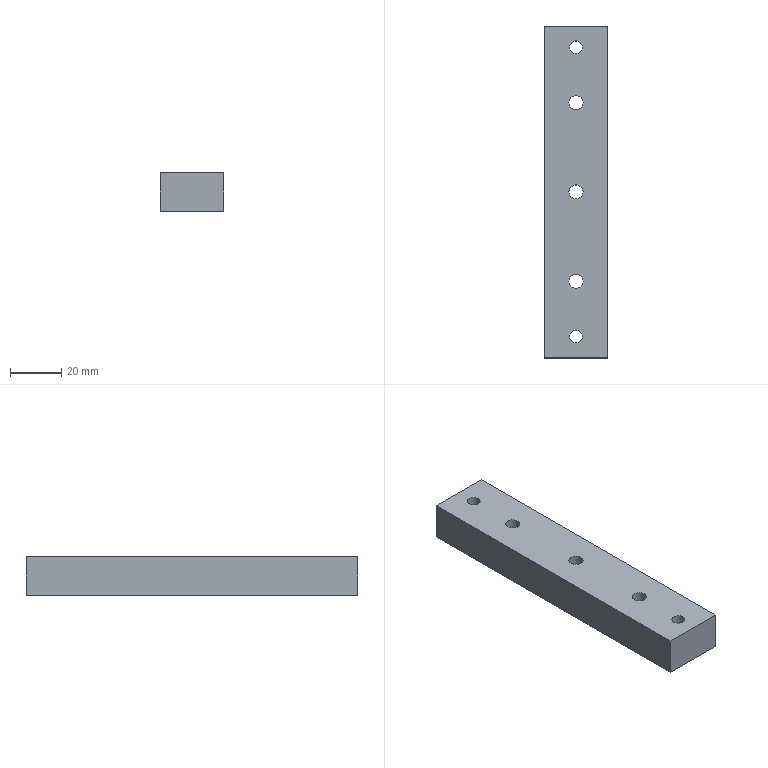Part | STEP file | 1 solid | 11 faces | box 25 x 130 x 15 mm | volume 47092 mm3 | plane 6 | cylinder 5 | commonest cylinder face diameters 5.5 x3 5 x2
STEP:
#1=CARTESIAN_POINT('',(0.,0.,0.));
#2=DIRECTION('',(0.,0.,1.));
#3=DIRECTION('',(1.,0.,0.));
#4=AXIS2_PLACEMENT_3D('',#1,#2,#3);
#5=CARTESIAN_POINT('',(1174.747,377.505,-51.381));
#6=VERTEX_POINT('',#5);
#7=CARTESIAN_POINT('',(1174.747,507.505,-51.381));
#8=VERTEX_POINT('',#7);
#9=CARTESIAN_POINT('',(1174.747,381.355,-51.381));
#10=DIRECTION('',(0.,1.,0.));
#11=VECTOR('',#10,1.);
#12=LINE('',#9,#11);
#13=CARTESIAN_POINT('',(1174.747,381.355,-48.381));
#14=DIRECTION('',(1.,0.,0.));
#15=DIRECTION('',(0.,0.,-1.));
#16=AXIS2_PLACEMENT_3D('',#13,#14,#15);
#17=PLANE('',#16);
#18=CARTESIAN_POINT('',(3.,0.));
#19=DIRECTION('',(0.,1.));
#20=VECTOR('',#19,1.);
#21=LINE('',#18,#20);
#22=(GEOMETRIC_REPRESENTATION_CONTEXT(2)PARAMETRIC_REPRESENTATION_CONTEXT()REPRESENTATION_CONTEXT('',''));
#23=DEFINITIONAL_REPRESENTATION('',(#21),#22);
#24=PCURVE('',#17,#23);
#25=CARTESIAN_POINT('',(18365.131,-3580.314,-51.381));
#26=DIRECTION('',(0.,0.,-1.));
#27=DIRECTION('',(-1.,0.,0.));
#28=AXIS2_PLACEMENT_3D('',#25,#26,#27);
#29=PLANE('',#28);
#30=CARTESIAN_POINT('',(17190.384,3961.669));
#31=DIRECTION('',(0.,1.));
#32=VECTOR('',#31,1.);
#33=LINE('',#30,#32);
#34=(GEOMETRIC_REPRESENTATION_CONTEXT(2)PARAMETRIC_REPRESENTATION_CONTEXT()REPRESENTATION_CONTEXT('',''));
#35=DEFINITIONAL_REPRESENTATION('',(#33),#34);
#36=PCURVE('',#29,#35);
#37=SURFACE_CURVE('',#12,(#24,#36),.PCURVE_S1.);
#38=EDGE_CURVE('',#6,#8,#37,.T.);
#39=ORIENTED_EDGE('',*,*,#38,.F.);
#40=CARTESIAN_POINT('',(1174.747,377.505,-36.381));
#41=VERTEX_POINT('',#40);
#42=CARTESIAN_POINT('',(1174.747,377.505,-48.381));
#43=DIRECTION('',(0.,0.,1.));
#44=VECTOR('',#43,1.);
#45=LINE('',#42,#44);
#46=CARTESIAN_POINT('',(0.,-3.85));
#47=DIRECTION('',(-1.,0.));
#48=VECTOR('',#47,1.);
#49=LINE('',#46,#48);
#50=(GEOMETRIC_REPRESENTATION_CONTEXT(2)PARAMETRIC_REPRESENTATION_CONTEXT()REPRESENTATION_CONTEXT('',''));
#51=DEFINITIONAL_REPRESENTATION('',(#49),#50);
#52=PCURVE('',#17,#51);
#53=CARTESIAN_POINT('',(1199.747,377.505,-48.381));
#54=DIRECTION('',(0.,1.,0.));
#55=DIRECTION('',(0.,0.,-1.));
#56=AXIS2_PLACEMENT_3D('',#53,#54,#55);
#57=PLANE('',#56);
#58=CARTESIAN_POINT('',(0.,25.));
#59=DIRECTION('',(-1.,0.));
#60=VECTOR('',#59,1.);
#61=LINE('',#58,#60);
#62=(GEOMETRIC_REPRESENTATION_CONTEXT(2)PARAMETRIC_REPRESENTATION_CONTEXT()REPRESENTATION_CONTEXT('',''));
#63=DEFINITIONAL_REPRESENTATION('',(#61),#62);
#64=PCURVE('',#57,#63);
#65=SURFACE_CURVE('',#45,(#52,#64),.PCURVE_S1.);
#66=EDGE_CURVE('',#6,#41,#65,.T.);
#67=ORIENTED_EDGE('',*,*,#66,.T.);
#68=CARTESIAN_POINT('',(1174.747,507.505,-36.381));
#69=VERTEX_POINT('',#68);
#70=CARTESIAN_POINT('',(1174.747,381.355,-36.381));
#71=DIRECTION('',(0.,1.,0.));
#72=VECTOR('',#71,1.);
#73=LINE('',#70,#72);
#74=CARTESIAN_POINT('',(-12.,0.));
#75=DIRECTION('',(0.,1.));
#76=VECTOR('',#75,1.);
#77=LINE('',#74,#76);
#78=(GEOMETRIC_REPRESENTATION_CONTEXT(2)PARAMETRIC_REPRESENTATION_CONTEXT()REPRESENTATION_CONTEXT('',''));
#79=DEFINITIONAL_REPRESENTATION('',(#77),#78);
#80=PCURVE('',#17,#79);
#81=CARTESIAN_POINT('',(18365.131,-3580.314,-36.381));
#82=DIRECTION('',(0.,0.,-1.));
#83=DIRECTION('',(-1.,0.,0.));
#84=AXIS2_PLACEMENT_3D('',#81,#82,#83);
#85=PLANE('',#84);
#86=CARTESIAN_POINT('',(17190.384,3961.669));
#87=DIRECTION('',(0.,1.));
#88=VECTOR('',#87,1.);
#89=LINE('',#86,#88);
#90=(GEOMETRIC_REPRESENTATION_CONTEXT(2)PARAMETRIC_REPRESENTATION_CONTEXT()REPRESENTATION_CONTEXT('',''));
#91=DEFINITIONAL_REPRESENTATION('',(#89),#90);
#92=PCURVE('',#85,#91);
#93=SURFACE_CURVE('',#73,(#80,#92),.PCURVE_S1.);
#94=EDGE_CURVE('',#41,#69,#93,.T.);
#95=ORIENTED_EDGE('',*,*,#94,.T.);
#96=CARTESIAN_POINT('',(1174.747,507.505,-48.381));
#97=DIRECTION('',(0.,0.,1.));
#98=VECTOR('',#97,1.);
#99=LINE('',#96,#98);
#100=CARTESIAN_POINT('',(0.,126.15));
#101=DIRECTION('',(-1.,0.));
#102=VECTOR('',#101,1.);
#103=LINE('',#100,#102);
#104=(GEOMETRIC_REPRESENTATION_CONTEXT(2)PARAMETRIC_REPRESENTATION_CONTEXT()REPRESENTATION_CONTEXT('',''));
#105=DEFINITIONAL_REPRESENTATION('',(#103),#104);
#106=PCURVE('',#17,#105);
#107=CARTESIAN_POINT('',(1174.747,507.505,-48.381));
#108=DIRECTION('',(0.,-1.,0.));
#109=DIRECTION('',(0.,0.,1.));
#110=AXIS2_PLACEMENT_3D('',#107,#108,#109);
#111=PLANE('',#110);
#112=CARTESIAN_POINT('',(0.,0.));
#113=DIRECTION('',(1.,0.));
#114=VECTOR('',#113,1.);
#115=LINE('',#112,#114);
#116=(GEOMETRIC_REPRESENTATION_CONTEXT(2)PARAMETRIC_REPRESENTATION_CONTEXT()REPRESENTATION_CONTEXT('',''));
#117=DEFINITIONAL_REPRESENTATION('',(#115),#116);
#118=PCURVE('',#111,#117);
#119=SURFACE_CURVE('',#99,(#106,#118),.PCURVE_S1.);
#120=EDGE_CURVE('',#8,#69,#119,.T.);
#121=ORIENTED_EDGE('',*,*,#120,.F.);
#122=EDGE_LOOP('',(#39,#67,#95,#121));
#123=FACE_BOUND('',#122,.T.);
#124=ADVANCED_FACE('',(#123),#17,.F.);
#125=CARTESIAN_POINT('',(1199.747,507.505,-36.381));
#126=VERTEX_POINT('',#125);
#127=CARTESIAN_POINT('',(1199.747,377.505,-36.381));
#128=VERTEX_POINT('',#127);
#129=CARTESIAN_POINT('',(1199.747,503.655,-36.381));
#130=DIRECTION('',(0.,-1.,0.));
#131=VECTOR('',#130,1.);
#132=LINE('',#129,#131);
#133=CARTESIAN_POINT('',(1199.747,503.655,-48.381));
#134=DIRECTION('',(-1.,0.,0.));
#135=DIRECTION('',(0.,0.,1.));
#136=AXIS2_PLACEMENT_3D('',#133,#134,#135);
#137=PLANE('',#136);
#138=CARTESIAN_POINT('',(12.,0.));
#139=DIRECTION('',(0.,-1.));
#140=VECTOR('',#139,1.);
#141=LINE('',#138,#140);
#142=(GEOMETRIC_REPRESENTATION_CONTEXT(2)PARAMETRIC_REPRESENTATION_CONTEXT()REPRESENTATION_CONTEXT('',''));
#143=DEFINITIONAL_REPRESENTATION('',(#141),#142);
#144=PCURVE('',#137,#143);
#145=CARTESIAN_POINT('',(17165.384,4083.969));
#146=DIRECTION('',(0.,-1.));
#147=VECTOR('',#146,1.);
#148=LINE('',#145,#147);
#149=(GEOMETRIC_REPRESENTATION_CONTEXT(2)PARAMETRIC_REPRESENTATION_CONTEXT()REPRESENTATION_CONTEXT('',''));
#150=DEFINITIONAL_REPRESENTATION('',(#148),#149);
#151=PCURVE('',#85,#150);
#152=SURFACE_CURVE('',#132,(#144,#151),.PCURVE_S1.);
#153=EDGE_CURVE('',#126,#128,#152,.T.);
#154=ORIENTED_EDGE('',*,*,#153,.T.);
#155=CARTESIAN_POINT('',(1199.747,377.505,-51.381));
#156=VERTEX_POINT('',#155);
#157=CARTESIAN_POINT('',(1199.747,377.505,-48.381));
#158=DIRECTION('',(0.,0.,1.));
#159=VECTOR('',#158,1.);
#160=LINE('',#157,#159);
#161=CARTESIAN_POINT('',(0.,-126.15));
#162=DIRECTION('',(1.,0.));
#163=VECTOR('',#162,1.);
#164=LINE('',#161,#163);
#165=(GEOMETRIC_REPRESENTATION_CONTEXT(2)PARAMETRIC_REPRESENTATION_CONTEXT()REPRESENTATION_CONTEXT('',''));
#166=DEFINITIONAL_REPRESENTATION('',(#164),#165);
#167=PCURVE('',#137,#166);
#168=CARTESIAN_POINT('',(0.,0.));
#169=DIRECTION('',(-1.,0.));
#170=VECTOR('',#169,1.);
#171=LINE('',#168,#170);
#172=(GEOMETRIC_REPRESENTATION_CONTEXT(2)PARAMETRIC_REPRESENTATION_CONTEXT()REPRESENTATION_CONTEXT('',''));
#173=DEFINITIONAL_REPRESENTATION('',(#171),#172);
#174=PCURVE('',#57,#173);
#175=SURFACE_CURVE('',#160,(#167,#174),.PCURVE_S1.);
#176=EDGE_CURVE('',#156,#128,#175,.T.);
#177=ORIENTED_EDGE('',*,*,#176,.F.);
#178=CARTESIAN_POINT('',(1199.747,507.505,-51.381));
#179=VERTEX_POINT('',#178);
#180=CARTESIAN_POINT('',(1199.747,503.655,-51.381));
#181=DIRECTION('',(0.,-1.,0.));
#182=VECTOR('',#181,1.);
#183=LINE('',#180,#182);
#184=CARTESIAN_POINT('',(-3.,0.));
#185=DIRECTION('',(0.,-1.));
#186=VECTOR('',#185,1.);
#187=LINE('',#184,#186);
#188=(GEOMETRIC_REPRESENTATION_CONTEXT(2)PARAMETRIC_REPRESENTATION_CONTEXT()REPRESENTATION_CONTEXT('',''));
#189=DEFINITIONAL_REPRESENTATION('',(#187),#188);
#190=PCURVE('',#137,#189);
#191=CARTESIAN_POINT('',(17165.384,4083.969));
#192=DIRECTION('',(0.,-1.));
#193=VECTOR('',#192,1.);
#194=LINE('',#191,#193);
#195=(GEOMETRIC_REPRESENTATION_CONTEXT(2)PARAMETRIC_REPRESENTATION_CONTEXT()REPRESENTATION_CONTEXT('',''));
#196=DEFINITIONAL_REPRESENTATION('',(#194),#195);
#197=PCURVE('',#29,#196);
#198=SURFACE_CURVE('',#183,(#190,#197),.PCURVE_S1.);
#199=EDGE_CURVE('',#179,#156,#198,.T.);
#200=ORIENTED_EDGE('',*,*,#199,.F.);
#201=CARTESIAN_POINT('',(1199.747,507.505,-48.381));
#202=DIRECTION('',(0.,0.,1.));
#203=VECTOR('',#202,1.);
#204=LINE('',#201,#203);
#205=CARTESIAN_POINT('',(0.,3.85));
#206=DIRECTION('',(1.,0.));
#207=VECTOR('',#206,1.);
#208=LINE('',#205,#207);
#209=(GEOMETRIC_REPRESENTATION_CONTEXT(2)PARAMETRIC_REPRESENTATION_CONTEXT()REPRESENTATION_CONTEXT('',''));
#210=DEFINITIONAL_REPRESENTATION('',(#208),#209);
#211=PCURVE('',#137,#210);
#212=CARTESIAN_POINT('',(0.,-25.));
#213=DIRECTION('',(1.,0.));
#214=VECTOR('',#213,1.);
#215=LINE('',#212,#214);
#216=(GEOMETRIC_REPRESENTATION_CONTEXT(2)PARAMETRIC_REPRESENTATION_CONTEXT()REPRESENTATION_CONTEXT('',''));
#217=DEFINITIONAL_REPRESENTATION('',(#215),#216);
#218=PCURVE('',#111,#217);
#219=SURFACE_CURVE('',#204,(#211,#218),.PCURVE_S1.);
#220=EDGE_CURVE('',#179,#126,#219,.T.);
#221=ORIENTED_EDGE('',*,*,#220,.T.);
#222=EDGE_LOOP('',(#154,#177,#200,#221));
#223=FACE_BOUND('',#222,.T.);
#224=ADVANCED_FACE('',(#223),#137,.F.);
#225=CARTESIAN_POINT('',(1184.747,385.855,-51.381));
#226=VERTEX_POINT('',#225);
#227=CARTESIAN_POINT('',(1187.247,385.855,-51.381));
#228=DIRECTION('',(0.,0.,1.));
#229=DIRECTION('',(-1.,0.,0.));
#230=AXIS2_PLACEMENT_3D('',#227,#228,#229);
#231=CIRCLE('',#230,2.5);
#232=CARTESIAN_POINT('',(17180.384,3966.169));
#233=CARTESIAN_POINT('',(17180.384,3961.839));
#234=CARTESIAN_POINT('',(17176.634,3964.004));
#235=CARTESIAN_POINT('',(17172.884,3966.169));
#236=CARTESIAN_POINT('',(17176.634,3968.334));
#237=CARTESIAN_POINT('',(17180.384,3970.499));
#238=CARTESIAN_POINT('',(17180.384,3966.169));
#239=(BOUNDED_CURVE()B_SPLINE_CURVE(2,(#232,#233,#234,#235,#236,#237,#238),.UNSPECIFIED.,.T.,.F.)B_SPLINE_CURVE_WITH_KNOTS((1,2,2,2,2,1),(-2.094,0.,2.094,4.189,6.283,8.378),.UNSPECIFIED.)CURVE()GEOMETRIC_REPRESENTATION_ITEM()RATIONAL_B_SPLINE_CURVE((1.,0.5,1.,0.5,1.,0.5,1.))REPRESENTATION_ITEM(''));
#240=(GEOMETRIC_REPRESENTATION_CONTEXT(2)PARAMETRIC_REPRESENTATION_CONTEXT()REPRESENTATION_CONTEXT('',''));
#241=DEFINITIONAL_REPRESENTATION('',(#239),#240);
#242=PCURVE('',#29,#241);
#243=CARTESIAN_POINT('',(1187.247,385.855,-30.381));
#244=DIRECTION('',(0.,0.,-1.));
#245=DIRECTION('',(-1.,0.,0.));
#246=AXIS2_PLACEMENT_3D('',#243,#244,#245);
#247=CYLINDRICAL_SURFACE('',#246,2.5);
#248=CARTESIAN_POINT('',(6.283,21.));
#249=DIRECTION('',(-1.,0.));
#250=VECTOR('',#249,1.);
#251=LINE('',#248,#250);
#252=(GEOMETRIC_REPRESENTATION_CONTEXT(2)PARAMETRIC_REPRESENTATION_CONTEXT()REPRESENTATION_CONTEXT('',''));
#253=DEFINITIONAL_REPRESENTATION('',(#251),#252);
#254=PCURVE('',#247,#253);
#255=SURFACE_CURVE('',#231,(#242,#254),.PCURVE_S1.);
#256=EDGE_CURVE('',#226,#226,#255,.T.);
#257=ORIENTED_EDGE('',*,*,#256,.T.);
#258=EDGE_LOOP('',(#257));
#259=FACE_BOUND('',#258,.T.);
#260=CARTESIAN_POINT('',(1184.747,499.155,-51.381));
#261=VERTEX_POINT('',#260);
#262=CARTESIAN_POINT('',(1187.247,499.155,-51.381));
#263=DIRECTION('',(0.,0.,1.));
#264=DIRECTION('',(-1.,0.,0.));
#265=AXIS2_PLACEMENT_3D('',#262,#263,#264);
#266=CIRCLE('',#265,2.5);
#267=CARTESIAN_POINT('',(17180.384,4079.469));
#268=CARTESIAN_POINT('',(17180.384,4075.139));
#269=CARTESIAN_POINT('',(17176.634,4077.304));
#270=CARTESIAN_POINT('',(17172.884,4079.469));
#271=CARTESIAN_POINT('',(17176.634,4081.634));
#272=CARTESIAN_POINT('',(17180.384,4083.799));
#273=CARTESIAN_POINT('',(17180.384,4079.469));
#274=(BOUNDED_CURVE()B_SPLINE_CURVE(2,(#267,#268,#269,#270,#271,#272,#273),.UNSPECIFIED.,.T.,.F.)B_SPLINE_CURVE_WITH_KNOTS((1,2,2,2,2,1),(-2.094,0.,2.094,4.189,6.283,8.378),.UNSPECIFIED.)CURVE()GEOMETRIC_REPRESENTATION_ITEM()RATIONAL_B_SPLINE_CURVE((1.,0.5,1.,0.5,1.,0.5,1.))REPRESENTATION_ITEM(''));
#275=(GEOMETRIC_REPRESENTATION_CONTEXT(2)PARAMETRIC_REPRESENTATION_CONTEXT()REPRESENTATION_CONTEXT('',''));
#276=DEFINITIONAL_REPRESENTATION('',(#274),#275);
#277=PCURVE('',#29,#276);
#278=CARTESIAN_POINT('',(1187.247,499.155,-30.381));
#279=DIRECTION('',(0.,0.,-1.));
#280=DIRECTION('',(-1.,0.,0.));
#281=AXIS2_PLACEMENT_3D('',#278,#279,#280);
#282=CYLINDRICAL_SURFACE('',#281,2.5);
#283=CARTESIAN_POINT('',(6.283,21.));
#284=DIRECTION('',(-1.,0.));
#285=VECTOR('',#284,1.);
#286=LINE('',#283,#285);
#287=(GEOMETRIC_REPRESENTATION_CONTEXT(2)PARAMETRIC_REPRESENTATION_CONTEXT()REPRESENTATION_CONTEXT('',''));
#288=DEFINITIONAL_REPRESENTATION('',(#286),#287);
#289=PCURVE('',#282,#288);
#290=SURFACE_CURVE('',#266,(#277,#289),.PCURVE_S1.);
#291=EDGE_CURVE('',#261,#261,#290,.T.);
#292=ORIENTED_EDGE('',*,*,#291,.T.);
#293=EDGE_LOOP('',(#292));
#294=FACE_BOUND('',#293,.T.);
#295=ORIENTED_EDGE('',*,*,#199,.T.);
#296=CARTESIAN_POINT('',(1199.747,377.505,-51.381));
#297=DIRECTION('',(-1.,0.,0.));
#298=VECTOR('',#297,1.);
#299=LINE('',#296,#298);
#300=CARTESIAN_POINT('',(17165.384,3957.819));
#301=DIRECTION('',(1.,0.));
#302=VECTOR('',#301,1.);
#303=LINE('',#300,#302);
#304=(GEOMETRIC_REPRESENTATION_CONTEXT(2)PARAMETRIC_REPRESENTATION_CONTEXT()REPRESENTATION_CONTEXT('',''));
#305=DEFINITIONAL_REPRESENTATION('',(#303),#304);
#306=PCURVE('',#29,#305);
#307=CARTESIAN_POINT('',(3.,0.));
#308=DIRECTION('',(0.,1.));
#309=VECTOR('',#308,1.);
#310=LINE('',#307,#309);
#311=(GEOMETRIC_REPRESENTATION_CONTEXT(2)PARAMETRIC_REPRESENTATION_CONTEXT()REPRESENTATION_CONTEXT('',''));
#312=DEFINITIONAL_REPRESENTATION('',(#310),#311);
#313=PCURVE('',#57,#312);
#314=SURFACE_CURVE('',#299,(#306,#313),.PCURVE_S1.);
#315=EDGE_CURVE('',#156,#6,#314,.T.);
#316=ORIENTED_EDGE('',*,*,#315,.T.);
#317=ORIENTED_EDGE('',*,*,#38,.T.);
#318=CARTESIAN_POINT('',(1174.747,507.505,-51.381));
#319=DIRECTION('',(1.,0.,0.));
#320=VECTOR('',#319,1.);
#321=LINE('',#318,#320);
#322=CARTESIAN_POINT('',(17190.384,4087.819));
#323=DIRECTION('',(-1.,0.));
#324=VECTOR('',#323,1.);
#325=LINE('',#322,#324);
#326=(GEOMETRIC_REPRESENTATION_CONTEXT(2)PARAMETRIC_REPRESENTATION_CONTEXT()REPRESENTATION_CONTEXT('',''));
#327=DEFINITIONAL_REPRESENTATION('',(#325),#326);
#328=PCURVE('',#29,#327);
#329=CARTESIAN_POINT('',(-3.,0.));
#330=DIRECTION('',(0.,-1.));
#331=VECTOR('',#330,1.);
#332=LINE('',#329,#331);
#333=(GEOMETRIC_REPRESENTATION_CONTEXT(2)PARAMETRIC_REPRESENTATION_CONTEXT()REPRESENTATION_CONTEXT('',''));
#334=DEFINITIONAL_REPRESENTATION('',(#332),#333);
#335=PCURVE('',#111,#334);
#336=SURFACE_CURVE('',#321,(#328,#335),.PCURVE_S1.);
#337=EDGE_CURVE('',#8,#179,#336,.T.);
#338=ORIENTED_EDGE('',*,*,#337,.T.);
#339=EDGE_LOOP('',(#295,#316,#317,#338));
#340=FACE_BOUND('',#339,.T.);
#341=CARTESIAN_POINT('',(1184.497,477.505,-51.381));
#342=VERTEX_POINT('',#341);
#343=CARTESIAN_POINT('',(1189.997,477.505,-51.381));
#344=VERTEX_POINT('',#343);
#345=CARTESIAN_POINT('',(1187.247,477.505,-51.381));
#346=DIRECTION('',(0.,0.,1.));
#347=DIRECTION('',(-1.,0.,0.));
#348=AXIS2_PLACEMENT_3D('',#345,#346,#347);
#349=CIRCLE('',#348,2.75);
#350=CARTESIAN_POINT('',(17180.634,4057.819));
#351=CARTESIAN_POINT('',(17180.634,4053.056));
#352=CARTESIAN_POINT('',(17176.509,4055.438));
#353=CARTESIAN_POINT('',(17172.384,4057.819));
#354=CARTESIAN_POINT('',(17176.509,4060.201));
#355=CARTESIAN_POINT('',(17180.634,4062.582));
#356=CARTESIAN_POINT('',(17180.634,4057.819));
#357=(BOUNDED_CURVE()B_SPLINE_CURVE(2,(#350,#351,#352,#353,#354,#355,#356),.UNSPECIFIED.,.T.,.F.)B_SPLINE_CURVE_WITH_KNOTS((1,2,2,2,2,1),(-2.094,0.,2.094,4.189,6.283,8.378),.UNSPECIFIED.)CURVE()GEOMETRIC_REPRESENTATION_ITEM()RATIONAL_B_SPLINE_CURVE((1.,0.5,1.,0.5,1.,0.5,1.))REPRESENTATION_ITEM(''));
#358=(GEOMETRIC_REPRESENTATION_CONTEXT(2)PARAMETRIC_REPRESENTATION_CONTEXT()REPRESENTATION_CONTEXT('',''));
#359=DEFINITIONAL_REPRESENTATION('',(#357),#358);
#360=PCURVE('',#29,#359);
#361=CARTESIAN_POINT('',(1187.247,477.505,-48.381));
#362=DIRECTION('',(0.,0.,1.));
#363=DIRECTION('',(1.,0.,0.));
#364=AXIS2_PLACEMENT_3D('',#361,#362,#363);
#365=CYLINDRICAL_SURFACE('',#364,2.75);
#366=CARTESIAN_POINT('',(3.142,-3.));
#367=DIRECTION('',(1.,0.));
#368=VECTOR('',#367,1.);
#369=LINE('',#366,#368);
#370=(GEOMETRIC_REPRESENTATION_CONTEXT(2)PARAMETRIC_REPRESENTATION_CONTEXT()REPRESENTATION_CONTEXT('',''));
#371=DEFINITIONAL_REPRESENTATION('',(#369),#370);
#372=PCURVE('',#365,#371);
#373=SURFACE_CURVE('',#349,(#360,#372),.PCURVE_S1.);
#374=EDGE_CURVE('',#342,#344,#373,.T.);
#375=ORIENTED_EDGE('',*,*,#374,.T.);
#376=CARTESIAN_POINT('',(1187.247,477.505,-51.381));
#377=DIRECTION('',(0.,0.,1.));
#378=DIRECTION('',(-1.,0.,0.));
#379=AXIS2_PLACEMENT_3D('',#376,#377,#378);
#380=CIRCLE('',#379,2.75);
#381=CARTESIAN_POINT('',(17180.634,4057.819));
#382=CARTESIAN_POINT('',(17180.634,4053.056));
#383=CARTESIAN_POINT('',(17176.509,4055.438));
#384=CARTESIAN_POINT('',(17172.384,4057.819));
#385=CARTESIAN_POINT('',(17176.509,4060.201));
#386=CARTESIAN_POINT('',(17180.634,4062.582));
#387=CARTESIAN_POINT('',(17180.634,4057.819));
#388=(BOUNDED_CURVE()B_SPLINE_CURVE(2,(#381,#382,#383,#384,#385,#386,#387),.UNSPECIFIED.,.T.,.F.)B_SPLINE_CURVE_WITH_KNOTS((1,2,2,2,2,1),(-2.094,0.,2.094,4.189,6.283,8.378),.UNSPECIFIED.)CURVE()GEOMETRIC_REPRESENTATION_ITEM()RATIONAL_B_SPLINE_CURVE((1.,0.5,1.,0.5,1.,0.5,1.))REPRESENTATION_ITEM(''));
#389=(GEOMETRIC_REPRESENTATION_CONTEXT(2)PARAMETRIC_REPRESENTATION_CONTEXT()REPRESENTATION_CONTEXT('',''));
#390=DEFINITIONAL_REPRESENTATION('',(#388),#389);
#391=PCURVE('',#29,#390);
#392=CARTESIAN_POINT('',(-3.142,-3.));
#393=DIRECTION('',(1.,0.));
#394=VECTOR('',#393,1.);
#395=LINE('',#392,#394);
#396=(GEOMETRIC_REPRESENTATION_CONTEXT(2)PARAMETRIC_REPRESENTATION_CONTEXT()REPRESENTATION_CONTEXT('',''));
#397=DEFINITIONAL_REPRESENTATION('',(#395),#396);
#398=PCURVE('',#365,#397);
#399=SURFACE_CURVE('',#380,(#391,#398),.PCURVE_S1.);
#400=EDGE_CURVE('',#344,#342,#399,.T.);
#401=ORIENTED_EDGE('',*,*,#400,.T.);
#402=EDGE_LOOP('',(#375,#401));
#403=FACE_BOUND('',#402,.T.);
#404=CARTESIAN_POINT('',(1184.497,442.505,-51.381));
#405=VERTEX_POINT('',#404);
#406=CARTESIAN_POINT('',(1189.997,442.505,-51.381));
#407=VERTEX_POINT('',#406);
#408=CARTESIAN_POINT('',(1187.247,442.505,-51.381));
#409=DIRECTION('',(0.,0.,1.));
#410=DIRECTION('',(-1.,0.,0.));
#411=AXIS2_PLACEMENT_3D('',#408,#409,#410);
#412=CIRCLE('',#411,2.75);
#413=CARTESIAN_POINT('',(17180.634,4022.819));
#414=CARTESIAN_POINT('',(17180.634,4018.056));
#415=CARTESIAN_POINT('',(17176.509,4020.438));
#416=CARTESIAN_POINT('',(17172.384,4022.819));
#417=CARTESIAN_POINT('',(17176.509,4025.201));
#418=CARTESIAN_POINT('',(17180.634,4027.582));
#419=CARTESIAN_POINT('',(17180.634,4022.819));
#420=(BOUNDED_CURVE()B_SPLINE_CURVE(2,(#413,#414,#415,#416,#417,#418,#419),.UNSPECIFIED.,.T.,.F.)B_SPLINE_CURVE_WITH_KNOTS((1,2,2,2,2,1),(-2.094,0.,2.094,4.189,6.283,8.378),.UNSPECIFIED.)CURVE()GEOMETRIC_REPRESENTATION_ITEM()RATIONAL_B_SPLINE_CURVE((1.,0.5,1.,0.5,1.,0.5,1.))REPRESENTATION_ITEM(''));
#421=(GEOMETRIC_REPRESENTATION_CONTEXT(2)PARAMETRIC_REPRESENTATION_CONTEXT()REPRESENTATION_CONTEXT('',''));
#422=DEFINITIONAL_REPRESENTATION('',(#420),#421);
#423=PCURVE('',#29,#422);
#424=CARTESIAN_POINT('',(1187.247,442.505,-48.381));
#425=DIRECTION('',(0.,0.,1.));
#426=DIRECTION('',(1.,0.,0.));
#427=AXIS2_PLACEMENT_3D('',#424,#425,#426);
#428=CYLINDRICAL_SURFACE('',#427,2.75);
#429=CARTESIAN_POINT('',(3.142,-3.));
#430=DIRECTION('',(1.,0.));
#431=VECTOR('',#430,1.);
#432=LINE('',#429,#431);
#433=(GEOMETRIC_REPRESENTATION_CONTEXT(2)PARAMETRIC_REPRESENTATION_CONTEXT()REPRESENTATION_CONTEXT('',''));
#434=DEFINITIONAL_REPRESENTATION('',(#432),#433);
#435=PCURVE('',#428,#434);
#436=SURFACE_CURVE('',#412,(#423,#435),.PCURVE_S1.);
#437=EDGE_CURVE('',#405,#407,#436,.T.);
#438=ORIENTED_EDGE('',*,*,#437,.T.);
#439=CARTESIAN_POINT('',(1187.247,442.505,-51.381));
#440=DIRECTION('',(0.,0.,1.));
#441=DIRECTION('',(-1.,0.,0.));
#442=AXIS2_PLACEMENT_3D('',#439,#440,#441);
#443=CIRCLE('',#442,2.75);
#444=CARTESIAN_POINT('',(17180.634,4022.819));
#445=CARTESIAN_POINT('',(17180.634,4018.056));
#446=CARTESIAN_POINT('',(17176.509,4020.438));
#447=CARTESIAN_POINT('',(17172.384,4022.819));
#448=CARTESIAN_POINT('',(17176.509,4025.201));
#449=CARTESIAN_POINT('',(17180.634,4027.582));
#450=CARTESIAN_POINT('',(17180.634,4022.819));
#451=(BOUNDED_CURVE()B_SPLINE_CURVE(2,(#444,#445,#446,#447,#448,#449,#450),.UNSPECIFIED.,.T.,.F.)B_SPLINE_CURVE_WITH_KNOTS((1,2,2,2,2,1),(-2.094,0.,2.094,4.189,6.283,8.378),.UNSPECIFIED.)CURVE()GEOMETRIC_REPRESENTATION_ITEM()RATIONAL_B_SPLINE_CURVE((1.,0.5,1.,0.5,1.,0.5,1.))REPRESENTATION_ITEM(''));
#452=(GEOMETRIC_REPRESENTATION_CONTEXT(2)PARAMETRIC_REPRESENTATION_CONTEXT()REPRESENTATION_CONTEXT('',''));
#453=DEFINITIONAL_REPRESENTATION('',(#451),#452);
#454=PCURVE('',#29,#453);
#455=CARTESIAN_POINT('',(-3.142,-3.));
#456=DIRECTION('',(1.,0.));
#457=VECTOR('',#456,1.);
#458=LINE('',#455,#457);
#459=(GEOMETRIC_REPRESENTATION_CONTEXT(2)PARAMETRIC_REPRESENTATION_CONTEXT()REPRESENTATION_CONTEXT('',''));
#460=DEFINITIONAL_REPRESENTATION('',(#458),#459);
#461=PCURVE('',#428,#460);
#462=SURFACE_CURVE('',#443,(#454,#461),.PCURVE_S1.);
#463=EDGE_CURVE('',#407,#405,#462,.T.);
#464=ORIENTED_EDGE('',*,*,#463,.T.);
#465=EDGE_LOOP('',(#438,#464));
#466=FACE_BOUND('',#465,.T.);
#467=CARTESIAN_POINT('',(1184.497,407.505,-51.381));
#468=VERTEX_POINT('',#467);
#469=CARTESIAN_POINT('',(1189.997,407.505,-51.381));
#470=VERTEX_POINT('',#469);
#471=CARTESIAN_POINT('',(1187.247,407.505,-51.381));
#472=DIRECTION('',(0.,0.,1.));
#473=DIRECTION('',(-1.,0.,0.));
#474=AXIS2_PLACEMENT_3D('',#471,#472,#473);
#475=CIRCLE('',#474,2.75);
#476=CARTESIAN_POINT('',(17180.634,3987.819));
#477=CARTESIAN_POINT('',(17180.634,3983.056));
#478=CARTESIAN_POINT('',(17176.509,3985.438));
#479=CARTESIAN_POINT('',(17172.384,3987.819));
#480=CARTESIAN_POINT('',(17176.509,3990.201));
#481=CARTESIAN_POINT('',(17180.634,3992.582));
#482=CARTESIAN_POINT('',(17180.634,3987.819));
#483=(BOUNDED_CURVE()B_SPLINE_CURVE(2,(#476,#477,#478,#479,#480,#481,#482),.UNSPECIFIED.,.T.,.F.)B_SPLINE_CURVE_WITH_KNOTS((1,2,2,2,2,1),(-2.094,0.,2.094,4.189,6.283,8.378),.UNSPECIFIED.)CURVE()GEOMETRIC_REPRESENTATION_ITEM()RATIONAL_B_SPLINE_CURVE((1.,0.5,1.,0.5,1.,0.5,1.))REPRESENTATION_ITEM(''));
#484=(GEOMETRIC_REPRESENTATION_CONTEXT(2)PARAMETRIC_REPRESENTATION_CONTEXT()REPRESENTATION_CONTEXT('',''));
#485=DEFINITIONAL_REPRESENTATION('',(#483),#484);
#486=PCURVE('',#29,#485);
#487=CARTESIAN_POINT('',(1187.247,407.505,-48.381));
#488=DIRECTION('',(0.,0.,1.));
#489=DIRECTION('',(1.,0.,0.));
#490=AXIS2_PLACEMENT_3D('',#487,#488,#489);
#491=CYLINDRICAL_SURFACE('',#490,2.75);
#492=CARTESIAN_POINT('',(3.142,-3.));
#493=DIRECTION('',(1.,0.));
#494=VECTOR('',#493,1.);
#495=LINE('',#492,#494);
#496=(GEOMETRIC_REPRESENTATION_CONTEXT(2)PARAMETRIC_REPRESENTATION_CONTEXT()REPRESENTATION_CONTEXT('',''));
#497=DEFINITIONAL_REPRESENTATION('',(#495),#496);
#498=PCURVE('',#491,#497);
#499=SURFACE_CURVE('',#475,(#486,#498),.PCURVE_S1.);
#500=EDGE_CURVE('',#468,#470,#499,.T.);
#501=ORIENTED_EDGE('',*,*,#500,.T.);
#502=CARTESIAN_POINT('',(1187.247,407.505,-51.381));
#503=DIRECTION('',(0.,0.,1.));
#504=DIRECTION('',(-1.,0.,0.));
#505=AXIS2_PLACEMENT_3D('',#502,#503,#504);
#506=CIRCLE('',#505,2.75);
#507=CARTESIAN_POINT('',(17180.634,3987.819));
#508=CARTESIAN_POINT('',(17180.634,3983.056));
#509=CARTESIAN_POINT('',(17176.509,3985.438));
#510=CARTESIAN_POINT('',(17172.384,3987.819));
#511=CARTESIAN_POINT('',(17176.509,3990.201));
#512=CARTESIAN_POINT('',(17180.634,3992.582));
#513=CARTESIAN_POINT('',(17180.634,3987.819));
#514=(BOUNDED_CURVE()B_SPLINE_CURVE(2,(#507,#508,#509,#510,#511,#512,#513),.UNSPECIFIED.,.T.,.F.)B_SPLINE_CURVE_WITH_KNOTS((1,2,2,2,2,1),(-2.094,0.,2.094,4.189,6.283,8.378),.UNSPECIFIED.)CURVE()GEOMETRIC_REPRESENTATION_ITEM()RATIONAL_B_SPLINE_CURVE((1.,0.5,1.,0.5,1.,0.5,1.))REPRESENTATION_ITEM(''));
#515=(GEOMETRIC_REPRESENTATION_CONTEXT(2)PARAMETRIC_REPRESENTATION_CONTEXT()REPRESENTATION_CONTEXT('',''));
#516=DEFINITIONAL_REPRESENTATION('',(#514),#515);
#517=PCURVE('',#29,#516);
#518=CARTESIAN_POINT('',(-3.142,-3.));
#519=DIRECTION('',(1.,0.));
#520=VECTOR('',#519,1.);
#521=LINE('',#518,#520);
#522=(GEOMETRIC_REPRESENTATION_CONTEXT(2)PARAMETRIC_REPRESENTATION_CONTEXT()REPRESENTATION_CONTEXT('',''));
#523=DEFINITIONAL_REPRESENTATION('',(#521),#522);
#524=PCURVE('',#491,#523);
#525=SURFACE_CURVE('',#506,(#517,#524),.PCURVE_S1.);
#526=EDGE_CURVE('',#470,#468,#525,.T.);
#527=ORIENTED_EDGE('',*,*,#526,.T.);
#528=EDGE_LOOP('',(#501,#527));
#529=FACE_BOUND('',#528,.T.);
#530=ADVANCED_FACE('',(#259,#294,#340,#403,#466,#529),#29,.T.);
#531=CARTESIAN_POINT('',(1184.747,385.855,-36.381));
#532=VERTEX_POINT('',#531);
#533=CARTESIAN_POINT('',(1187.247,385.855,-36.381));
#534=DIRECTION('',(0.,0.,1.));
#535=DIRECTION('',(-1.,0.,0.));
#536=AXIS2_PLACEMENT_3D('',#533,#534,#535);
#537=CIRCLE('',#536,2.5);
#538=CARTESIAN_POINT('',(17180.384,3966.169));
#539=CARTESIAN_POINT('',(17180.384,3961.839));
#540=CARTESIAN_POINT('',(17176.634,3964.004));
#541=CARTESIAN_POINT('',(17172.884,3966.169));
#542=CARTESIAN_POINT('',(17176.634,3968.334));
#543=CARTESIAN_POINT('',(17180.384,3970.499));
#544=CARTESIAN_POINT('',(17180.384,3966.169));
#545=(BOUNDED_CURVE()B_SPLINE_CURVE(2,(#538,#539,#540,#541,#542,#543,#544),.UNSPECIFIED.,.T.,.F.)B_SPLINE_CURVE_WITH_KNOTS((1,2,2,2,2,1),(-2.094,0.,2.094,4.189,6.283,8.378),.UNSPECIFIED.)CURVE()GEOMETRIC_REPRESENTATION_ITEM()RATIONAL_B_SPLINE_CURVE((1.,0.5,1.,0.5,1.,0.5,1.))REPRESENTATION_ITEM(''));
#546=(GEOMETRIC_REPRESENTATION_CONTEXT(2)PARAMETRIC_REPRESENTATION_CONTEXT()REPRESENTATION_CONTEXT('',''));
#547=DEFINITIONAL_REPRESENTATION('',(#545),#546);
#548=PCURVE('',#85,#547);
#549=CARTESIAN_POINT('',(6.283,6.));
#550=DIRECTION('',(-1.,0.));
#551=VECTOR('',#550,1.);
#552=LINE('',#549,#551);
#553=(GEOMETRIC_REPRESENTATION_CONTEXT(2)PARAMETRIC_REPRESENTATION_CONTEXT()REPRESENTATION_CONTEXT('',''));
#554=DEFINITIONAL_REPRESENTATION('',(#552),#553);
#555=PCURVE('',#247,#554);
#556=SURFACE_CURVE('',#537,(#548,#555),.PCURVE_S1.);
#557=EDGE_CURVE('',#532,#532,#556,.T.);
#558=ORIENTED_EDGE('',*,*,#557,.F.);
#559=EDGE_LOOP('',(#558));
#560=FACE_BOUND('',#559,.T.);
#561=CARTESIAN_POINT('',(1184.747,499.155,-36.381));
#562=VERTEX_POINT('',#561);
#563=CARTESIAN_POINT('',(1187.247,499.155,-36.381));
#564=DIRECTION('',(0.,0.,1.));
#565=DIRECTION('',(-1.,0.,0.));
#566=AXIS2_PLACEMENT_3D('',#563,#564,#565);
#567=CIRCLE('',#566,2.5);
#568=CARTESIAN_POINT('',(17180.384,4079.469));
#569=CARTESIAN_POINT('',(17180.384,4075.139));
#570=CARTESIAN_POINT('',(17176.634,4077.304));
#571=CARTESIAN_POINT('',(17172.884,4079.469));
#572=CARTESIAN_POINT('',(17176.634,4081.634));
#573=CARTESIAN_POINT('',(17180.384,4083.799));
#574=CARTESIAN_POINT('',(17180.384,4079.469));
#575=(BOUNDED_CURVE()B_SPLINE_CURVE(2,(#568,#569,#570,#571,#572,#573,#574),.UNSPECIFIED.,.T.,.F.)B_SPLINE_CURVE_WITH_KNOTS((1,2,2,2,2,1),(-2.094,0.,2.094,4.189,6.283,8.378),.UNSPECIFIED.)CURVE()GEOMETRIC_REPRESENTATION_ITEM()RATIONAL_B_SPLINE_CURVE((1.,0.5,1.,0.5,1.,0.5,1.))REPRESENTATION_ITEM(''));
#576=(GEOMETRIC_REPRESENTATION_CONTEXT(2)PARAMETRIC_REPRESENTATION_CONTEXT()REPRESENTATION_CONTEXT('',''));
#577=DEFINITIONAL_REPRESENTATION('',(#575),#576);
#578=PCURVE('',#85,#577);
#579=CARTESIAN_POINT('',(6.283,6.));
#580=DIRECTION('',(-1.,0.));
#581=VECTOR('',#580,1.);
#582=LINE('',#579,#581);
#583=(GEOMETRIC_REPRESENTATION_CONTEXT(2)PARAMETRIC_REPRESENTATION_CONTEXT()REPRESENTATION_CONTEXT('',''));
#584=DEFINITIONAL_REPRESENTATION('',(#582),#583);
#585=PCURVE('',#282,#584);
#586=SURFACE_CURVE('',#567,(#578,#585),.PCURVE_S1.);
#587=EDGE_CURVE('',#562,#562,#586,.T.);
#588=ORIENTED_EDGE('',*,*,#587,.F.);
#589=EDGE_LOOP('',(#588));
#590=FACE_BOUND('',#589,.T.);
#591=CARTESIAN_POINT('',(1189.997,442.505,-36.381));
#592=VERTEX_POINT('',#591);
#593=CARTESIAN_POINT('',(1187.247,442.505,-36.381));
#594=DIRECTION('',(0.,0.,-1.));
#595=DIRECTION('',(1.,0.,0.));
#596=AXIS2_PLACEMENT_3D('',#593,#594,#595);
#597=CIRCLE('',#596,2.75);
#598=CARTESIAN_POINT('',(17177.884,4022.819));
#599=DIRECTION('',(-1.,0.));
#600=AXIS2_PLACEMENT_2D('',#598,#599);
#601=CIRCLE('',#600,2.75);
#602=(GEOMETRIC_REPRESENTATION_CONTEXT(2)PARAMETRIC_REPRESENTATION_CONTEXT()REPRESENTATION_CONTEXT('',''));
#603=DEFINITIONAL_REPRESENTATION('',(#601),#602);
#604=PCURVE('',#85,#603);
#605=CARTESIAN_POINT('',(6.283,12.));
#606=DIRECTION('',(-1.,0.));
#607=VECTOR('',#606,1.);
#608=LINE('',#605,#607);
#609=(GEOMETRIC_REPRESENTATION_CONTEXT(2)PARAMETRIC_REPRESENTATION_CONTEXT()REPRESENTATION_CONTEXT('',''));
#610=DEFINITIONAL_REPRESENTATION('',(#608),#609);
#611=PCURVE('',#428,#610);
#612=SURFACE_CURVE('',#597,(#604,#611),.PCURVE_S1.);
#613=EDGE_CURVE('',#592,#592,#612,.T.);
#614=ORIENTED_EDGE('',*,*,#613,.T.);
#615=EDGE_LOOP('',(#614));
#616=FACE_BOUND('',#615,.T.);
#617=CARTESIAN_POINT('',(1189.997,477.505,-36.381));
#618=VERTEX_POINT('',#617);
#619=CARTESIAN_POINT('',(1187.247,477.505,-36.381));
#620=DIRECTION('',(0.,0.,-1.));
#621=DIRECTION('',(1.,0.,0.));
#622=AXIS2_PLACEMENT_3D('',#619,#620,#621);
#623=CIRCLE('',#622,2.75);
#624=CARTESIAN_POINT('',(17177.884,4057.819));
#625=DIRECTION('',(-1.,0.));
#626=AXIS2_PLACEMENT_2D('',#624,#625);
#627=CIRCLE('',#626,2.75);
#628=(GEOMETRIC_REPRESENTATION_CONTEXT(2)PARAMETRIC_REPRESENTATION_CONTEXT()REPRESENTATION_CONTEXT('',''));
#629=DEFINITIONAL_REPRESENTATION('',(#627),#628);
#630=PCURVE('',#85,#629);
#631=CARTESIAN_POINT('',(6.283,12.));
#632=DIRECTION('',(-1.,0.));
#633=VECTOR('',#632,1.);
#634=LINE('',#631,#633);
#635=(GEOMETRIC_REPRESENTATION_CONTEXT(2)PARAMETRIC_REPRESENTATION_CONTEXT()REPRESENTATION_CONTEXT('',''));
#636=DEFINITIONAL_REPRESENTATION('',(#634),#635);
#637=PCURVE('',#365,#636);
#638=SURFACE_CURVE('',#623,(#630,#637),.PCURVE_S1.);
#639=EDGE_CURVE('',#618,#618,#638,.T.);
#640=ORIENTED_EDGE('',*,*,#639,.T.);
#641=EDGE_LOOP('',(#640));
#642=FACE_BOUND('',#641,.T.);
#643=CARTESIAN_POINT('',(1199.747,377.505,-36.381));
#644=DIRECTION('',(-1.,0.,0.));
#645=VECTOR('',#644,1.);
#646=LINE('',#643,#645);
#647=CARTESIAN_POINT('',(17165.384,3957.819));
#648=DIRECTION('',(1.,0.));
#649=VECTOR('',#648,1.);
#650=LINE('',#647,#649);
#651=(GEOMETRIC_REPRESENTATION_CONTEXT(2)PARAMETRIC_REPRESENTATION_CONTEXT()REPRESENTATION_CONTEXT('',''));
#652=DEFINITIONAL_REPRESENTATION('',(#650),#651);
#653=PCURVE('',#85,#652);
#654=CARTESIAN_POINT('',(-12.,0.));
#655=DIRECTION('',(0.,1.));
#656=VECTOR('',#655,1.);
#657=LINE('',#654,#656);
#658=(GEOMETRIC_REPRESENTATION_CONTEXT(2)PARAMETRIC_REPRESENTATION_CONTEXT()REPRESENTATION_CONTEXT('',''));
#659=DEFINITIONAL_REPRESENTATION('',(#657),#658);
#660=PCURVE('',#57,#659);
#661=SURFACE_CURVE('',#646,(#653,#660),.PCURVE_S1.);
#662=EDGE_CURVE('',#128,#41,#661,.T.);
#663=ORIENTED_EDGE('',*,*,#662,.F.);
#664=ORIENTED_EDGE('',*,*,#153,.F.);
#665=CARTESIAN_POINT('',(1174.747,507.505,-36.381));
#666=DIRECTION('',(1.,0.,0.));
#667=VECTOR('',#666,1.);
#668=LINE('',#665,#667);
#669=CARTESIAN_POINT('',(17190.384,4087.819));
#670=DIRECTION('',(-1.,0.));
#671=VECTOR('',#670,1.);
#672=LINE('',#669,#671);
#673=(GEOMETRIC_REPRESENTATION_CONTEXT(2)PARAMETRIC_REPRESENTATION_CONTEXT()REPRESENTATION_CONTEXT('',''));
#674=DEFINITIONAL_REPRESENTATION('',(#672),#673);
#675=PCURVE('',#85,#674);
#676=CARTESIAN_POINT('',(12.,0.));
#677=DIRECTION('',(0.,-1.));
#678=VECTOR('',#677,1.);
#679=LINE('',#676,#678);
#680=(GEOMETRIC_REPRESENTATION_CONTEXT(2)PARAMETRIC_REPRESENTATION_CONTEXT()REPRESENTATION_CONTEXT('',''));
#681=DEFINITIONAL_REPRESENTATION('',(#679),#680);
#682=PCURVE('',#111,#681);
#683=SURFACE_CURVE('',#668,(#675,#682),.PCURVE_S1.);
#684=EDGE_CURVE('',#69,#126,#683,.T.);
#685=ORIENTED_EDGE('',*,*,#684,.F.);
#686=ORIENTED_EDGE('',*,*,#94,.F.);
#687=EDGE_LOOP('',(#663,#664,#685,#686));
#688=FACE_BOUND('',#687,.T.);
#689=CARTESIAN_POINT('',(1189.997,407.505,-36.381));
#690=VERTEX_POINT('',#689);
#691=CARTESIAN_POINT('',(1187.247,407.505,-36.381));
#692=DIRECTION('',(0.,0.,-1.));
#693=DIRECTION('',(1.,0.,0.));
#694=AXIS2_PLACEMENT_3D('',#691,#692,#693);
#695=CIRCLE('',#694,2.75);
#696=CARTESIAN_POINT('',(17177.884,3987.819));
#697=DIRECTION('',(-1.,0.));
#698=AXIS2_PLACEMENT_2D('',#696,#697);
#699=CIRCLE('',#698,2.75);
#700=(GEOMETRIC_REPRESENTATION_CONTEXT(2)PARAMETRIC_REPRESENTATION_CONTEXT()REPRESENTATION_CONTEXT('',''));
#701=DEFINITIONAL_REPRESENTATION('',(#699),#700);
#702=PCURVE('',#85,#701);
#703=CARTESIAN_POINT('',(6.283,12.));
#704=DIRECTION('',(-1.,0.));
#705=VECTOR('',#704,1.);
#706=LINE('',#703,#705);
#707=(GEOMETRIC_REPRESENTATION_CONTEXT(2)PARAMETRIC_REPRESENTATION_CONTEXT()REPRESENTATION_CONTEXT('',''));
#708=DEFINITIONAL_REPRESENTATION('',(#706),#707);
#709=PCURVE('',#491,#708);
#710=SURFACE_CURVE('',#695,(#702,#709),.PCURVE_S1.);
#711=EDGE_CURVE('',#690,#690,#710,.T.);
#712=ORIENTED_EDGE('',*,*,#711,.T.);
#713=EDGE_LOOP('',(#712));
#714=FACE_BOUND('',#713,.T.);
#715=ADVANCED_FACE('',(#560,#590,#616,#642,#688,#714),#85,.F.);
#716=ORIENTED_EDGE('',*,*,#613,.T.);
#717=CARTESIAN_POINT('',(1189.997,442.505,-51.381));
#718=CARTESIAN_POINT('',(1189.997,442.505,-36.381));
#719=B_SPLINE_CURVE_WITH_KNOTS('',1,(#717,#718),.UNSPECIFIED.,.F.,.F.,(2,2),(-3.,12.),.PIECEWISE_BEZIER_KNOTS.);
#720=CARTESIAN_POINT('',(0.,0.));
#721=DIRECTION('',(0.,1.));
#722=VECTOR('',#721,1.);
#723=LINE('',#720,#722);
#724=(GEOMETRIC_REPRESENTATION_CONTEXT(2)PARAMETRIC_REPRESENTATION_CONTEXT()REPRESENTATION_CONTEXT('',''));
#725=DEFINITIONAL_REPRESENTATION('',(#723),#724);
#726=PCURVE('',#428,#725);
#727=CARTESIAN_POINT('',(6.283,0.));
#728=DIRECTION('',(0.,1.));
#729=VECTOR('',#728,1.);
#730=LINE('',#727,#729);
#731=(GEOMETRIC_REPRESENTATION_CONTEXT(2)PARAMETRIC_REPRESENTATION_CONTEXT()REPRESENTATION_CONTEXT('',''));
#732=DEFINITIONAL_REPRESENTATION('',(#730),#731);
#733=PCURVE('',#428,#732);
#734=SEAM_CURVE('',#719,(#726,#733),.PCURVE_S1.);
#735=EDGE_CURVE('',#407,#592,#734,.T.);
#736=ORIENTED_EDGE('',*,*,#735,.F.);
#737=ORIENTED_EDGE('',*,*,#463,.T.);
#738=ORIENTED_EDGE('',*,*,#437,.T.);
#739=ORIENTED_EDGE('',*,*,#735,.T.);
#740=EDGE_LOOP('',(#716,#736,#737,#738,#739));
#741=FACE_BOUND('',#740,.F.);
#742=ADVANCED_FACE('',(#741),#428,.F.);
#743=ORIENTED_EDGE('',*,*,#684,.T.);
#744=ORIENTED_EDGE('',*,*,#220,.F.);
#745=ORIENTED_EDGE('',*,*,#337,.F.);
#746=ORIENTED_EDGE('',*,*,#120,.T.);
#747=EDGE_LOOP('',(#743,#744,#745,#746));
#748=FACE_BOUND('',#747,.T.);
#749=ADVANCED_FACE('',(#748),#111,.F.);
#750=ORIENTED_EDGE('',*,*,#374,.T.);
#751=CARTESIAN_POINT('',(1189.997,477.505,-51.381));
#752=CARTESIAN_POINT('',(1189.997,477.505,-36.381));
#753=B_SPLINE_CURVE_WITH_KNOTS('',1,(#751,#752),.UNSPECIFIED.,.F.,.F.,(2,2),(-3.,12.),.PIECEWISE_BEZIER_KNOTS.);
#754=CARTESIAN_POINT('',(6.283,0.));
#755=DIRECTION('',(0.,1.));
#756=VECTOR('',#755,1.);
#757=LINE('',#754,#756);
#758=(GEOMETRIC_REPRESENTATION_CONTEXT(2)PARAMETRIC_REPRESENTATION_CONTEXT()REPRESENTATION_CONTEXT('',''));
#759=DEFINITIONAL_REPRESENTATION('',(#757),#758);
#760=PCURVE('',#365,#759);
#761=CARTESIAN_POINT('',(0.,0.));
#762=DIRECTION('',(0.,1.));
#763=VECTOR('',#762,1.);
#764=LINE('',#761,#763);
#765=(GEOMETRIC_REPRESENTATION_CONTEXT(2)PARAMETRIC_REPRESENTATION_CONTEXT()REPRESENTATION_CONTEXT('',''));
#766=DEFINITIONAL_REPRESENTATION('',(#764),#765);
#767=PCURVE('',#365,#766);
#768=SEAM_CURVE('',#753,(#760,#767),.PCURVE_S1.);
#769=EDGE_CURVE('',#344,#618,#768,.T.);
#770=ORIENTED_EDGE('',*,*,#769,.T.);
#771=ORIENTED_EDGE('',*,*,#639,.T.);
#772=ORIENTED_EDGE('',*,*,#769,.F.);
#773=ORIENTED_EDGE('',*,*,#400,.T.);
#774=EDGE_LOOP('',(#750,#770,#771,#772,#773));
#775=FACE_BOUND('',#774,.F.);
#776=ADVANCED_FACE('',(#775),#365,.F.);
#777=ORIENTED_EDGE('',*,*,#500,.T.);
#778=CARTESIAN_POINT('',(1189.997,407.505,-51.381));
#779=CARTESIAN_POINT('',(1189.997,407.505,-36.381));
#780=B_SPLINE_CURVE_WITH_KNOTS('',1,(#778,#779),.UNSPECIFIED.,.F.,.F.,(2,2),(-3.,12.),.PIECEWISE_BEZIER_KNOTS.);
#781=CARTESIAN_POINT('',(6.283,0.));
#782=DIRECTION('',(0.,1.));
#783=VECTOR('',#782,1.);
#784=LINE('',#781,#783);
#785=(GEOMETRIC_REPRESENTATION_CONTEXT(2)PARAMETRIC_REPRESENTATION_CONTEXT()REPRESENTATION_CONTEXT('',''));
#786=DEFINITIONAL_REPRESENTATION('',(#784),#785);
#787=PCURVE('',#491,#786);
#788=CARTESIAN_POINT('',(0.,0.));
#789=DIRECTION('',(0.,1.));
#790=VECTOR('',#789,1.);
#791=LINE('',#788,#790);
#792=(GEOMETRIC_REPRESENTATION_CONTEXT(2)PARAMETRIC_REPRESENTATION_CONTEXT()REPRESENTATION_CONTEXT('',''));
#793=DEFINITIONAL_REPRESENTATION('',(#791),#792);
#794=PCURVE('',#491,#793);
#795=SEAM_CURVE('',#780,(#787,#794),.PCURVE_S1.);
#796=EDGE_CURVE('',#470,#690,#795,.T.);
#797=ORIENTED_EDGE('',*,*,#796,.T.);
#798=ORIENTED_EDGE('',*,*,#711,.T.);
#799=ORIENTED_EDGE('',*,*,#796,.F.);
#800=ORIENTED_EDGE('',*,*,#526,.T.);
#801=EDGE_LOOP('',(#777,#797,#798,#799,#800));
#802=FACE_BOUND('',#801,.F.);
#803=ADVANCED_FACE('',(#802),#491,.F.);
#804=ORIENTED_EDGE('',*,*,#662,.T.);
#805=ORIENTED_EDGE('',*,*,#66,.F.);
#806=ORIENTED_EDGE('',*,*,#315,.F.);
#807=ORIENTED_EDGE('',*,*,#176,.T.);
#808=EDGE_LOOP('',(#804,#805,#806,#807));
#809=FACE_BOUND('',#808,.T.);
#810=ADVANCED_FACE('',(#809),#57,.F.);
#811=ORIENTED_EDGE('',*,*,#291,.T.);
#812=CARTESIAN_POINT('',(1184.747,499.155,-36.381));
#813=CARTESIAN_POINT('',(1184.747,499.155,-51.381));
#814=B_SPLINE_CURVE_WITH_KNOTS('',1,(#812,#813),.UNSPECIFIED.,.F.,.F.,(2,2),(6.,21.),.PIECEWISE_BEZIER_KNOTS.);
#815=CARTESIAN_POINT('',(0.,0.));
#816=DIRECTION('',(0.,1.));
#817=VECTOR('',#816,1.);
#818=LINE('',#815,#817);
#819=(GEOMETRIC_REPRESENTATION_CONTEXT(2)PARAMETRIC_REPRESENTATION_CONTEXT()REPRESENTATION_CONTEXT('',''));
#820=DEFINITIONAL_REPRESENTATION('',(#818),#819);
#821=PCURVE('',#282,#820);
#822=CARTESIAN_POINT('',(6.283,0.));
#823=DIRECTION('',(0.,1.));
#824=VECTOR('',#823,1.);
#825=LINE('',#822,#824);
#826=(GEOMETRIC_REPRESENTATION_CONTEXT(2)PARAMETRIC_REPRESENTATION_CONTEXT()REPRESENTATION_CONTEXT('',''));
#827=DEFINITIONAL_REPRESENTATION('',(#825),#826);
#828=PCURVE('',#282,#827);
#829=SEAM_CURVE('',#814,(#821,#828),.PCURVE_S1.);
#830=EDGE_CURVE('',#562,#261,#829,.T.);
#831=ORIENTED_EDGE('',*,*,#830,.F.);
#832=ORIENTED_EDGE('',*,*,#587,.F.);
#833=ORIENTED_EDGE('',*,*,#830,.T.);
#834=EDGE_LOOP('',(#811,#831,#832,#833));
#835=FACE_BOUND('',#834,.F.);
#836=ADVANCED_FACE('',(#835),#282,.F.);
#837=ORIENTED_EDGE('',*,*,#256,.T.);
#838=CARTESIAN_POINT('',(1184.747,385.855,-36.381));
#839=CARTESIAN_POINT('',(1184.747,385.855,-51.381));
#840=B_SPLINE_CURVE_WITH_KNOTS('',1,(#838,#839),.UNSPECIFIED.,.F.,.F.,(2,2),(6.,21.),.PIECEWISE_BEZIER_KNOTS.);
#841=CARTESIAN_POINT('',(0.,0.));
#842=DIRECTION('',(0.,1.));
#843=VECTOR('',#842,1.);
#844=LINE('',#841,#843);
#845=(GEOMETRIC_REPRESENTATION_CONTEXT(2)PARAMETRIC_REPRESENTATION_CONTEXT()REPRESENTATION_CONTEXT('',''));
#846=DEFINITIONAL_REPRESENTATION('',(#844),#845);
#847=PCURVE('',#247,#846);
#848=CARTESIAN_POINT('',(6.283,0.));
#849=DIRECTION('',(0.,1.));
#850=VECTOR('',#849,1.);
#851=LINE('',#848,#850);
#852=(GEOMETRIC_REPRESENTATION_CONTEXT(2)PARAMETRIC_REPRESENTATION_CONTEXT()REPRESENTATION_CONTEXT('',''));
#853=DEFINITIONAL_REPRESENTATION('',(#851),#852);
#854=PCURVE('',#247,#853);
#855=SEAM_CURVE('',#840,(#847,#854),.PCURVE_S1.);
#856=EDGE_CURVE('',#532,#226,#855,.T.);
#857=ORIENTED_EDGE('',*,*,#856,.F.);
#858=ORIENTED_EDGE('',*,*,#557,.F.);
#859=ORIENTED_EDGE('',*,*,#856,.T.);
#860=EDGE_LOOP('',(#837,#857,#858,#859));
#861=FACE_BOUND('',#860,.F.);
#862=ADVANCED_FACE('',(#861),#247,.F.);
#863=CLOSED_SHELL('',(#124,#224,#530,#715,#742,#749,#776,#803,#810,#836,#862));
#864=MANIFOLD_SOLID_BREP('',#863);
#865=(LENGTH_UNIT()NAMED_UNIT(*)SI_UNIT(.MILLI.,.METRE.));
#866=UNCERTAINTY_MEASURE_WITH_UNIT(LENGTH_MEASURE(0.000005),#865,'','');
#867=(NAMED_UNIT(*)PLANE_ANGLE_UNIT()SI_UNIT($,.RADIAN.));
#868=(NAMED_UNIT(*)SI_UNIT($,.STERADIAN.)SOLID_ANGLE_UNIT());
#869=(GEOMETRIC_REPRESENTATION_CONTEXT(3)GLOBAL_UNCERTAINTY_ASSIGNED_CONTEXT((#866))GLOBAL_UNIT_ASSIGNED_CONTEXT((#865,#867,#868))REPRESENTATION_CONTEXT('',''));
#870=ADVANCED_BREP_SHAPE_REPRESENTATION('',(#4,#864),#869);